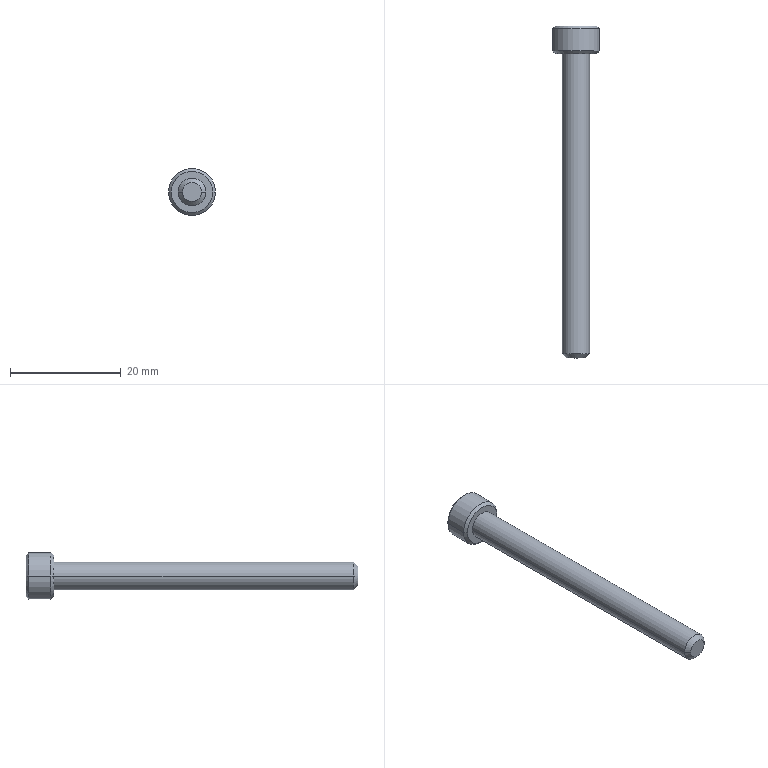Part | STEP file | BB62-M5-55L | 1 solid | 27 faces | box 8.5 x 60 x 8.5 mm | volume 1311 mm3 | plane 15 | cone 8 | cylinder 4 | commonest cylinder face diameters 5 x2 8.5 x2
STEP:
#1=CARTESIAN_POINT('',(0.,1.178,0.));
#2=VERTEX_POINT('',#1);
#3=CARTESIAN_POINT('',(2.29,2.5,0.));
#4=VERTEX_POINT('',#3);
#5=CARTESIAN_POINT('',(0.,1.178,0.));
#6=DIRECTION('',(0.866,0.5,0.));
#7=VECTOR('',#6,1000.);
#8=LINE('',#5,#7);
#9=EDGE_CURVE('',#2,#4,#8,.T.);
#10=ORIENTED_EDGE('',*,*,#9,.F.);
#11=CARTESIAN_POINT('',(-2.29,2.5,0.));
#12=VERTEX_POINT('',#11);
#13=CARTESIAN_POINT('',(0.,1.178,0.));
#14=DIRECTION('',(-0.866,0.5,0.));
#15=VECTOR('',#14,1000.);
#16=LINE('',#13,#15);
#17=EDGE_CURVE('',#2,#12,#16,.T.);
#18=ORIENTED_EDGE('',*,*,#17,.T.);
#19=CARTESIAN_POINT('',(-1.983,2.5,1.145));
#20=VERTEX_POINT('',#19);
#21=CARTESIAN_POINT('',(0.,2.5,0.));
#22=DIRECTION('',(0.,-1.,0.));
#23=DIRECTION('',(-1.,0.,0.));
#24=AXIS2_PLACEMENT_3D('',#21,#22,#23);
#25=CIRCLE('',#24,2.29);
#26=EDGE_CURVE('',#20,#12,#25,.T.);
#27=ORIENTED_EDGE('',*,*,#26,.F.);
#28=CARTESIAN_POINT('',(0.,2.5,2.29));
#29=VERTEX_POINT('',#28);
#30=CARTESIAN_POINT('',(0.,2.5,0.));
#31=DIRECTION('',(0.,-1.,0.));
#32=DIRECTION('',(-1.,0.,0.));
#33=AXIS2_PLACEMENT_3D('',#30,#31,#32);
#34=CIRCLE('',#33,2.29);
#35=EDGE_CURVE('',#29,#20,#34,.T.);
#36=ORIENTED_EDGE('',*,*,#35,.F.);
#37=CARTESIAN_POINT('',(1.983,2.5,1.145));
#38=VERTEX_POINT('',#37);
#39=CARTESIAN_POINT('',(0.,2.5,0.));
#40=DIRECTION('',(0.,-1.,0.));
#41=DIRECTION('',(-1.,0.,0.));
#42=AXIS2_PLACEMENT_3D('',#39,#40,#41);
#43=CIRCLE('',#42,2.29);
#44=EDGE_CURVE('',#38,#29,#43,.T.);
#45=ORIENTED_EDGE('',*,*,#44,.F.);
#46=CARTESIAN_POINT('',(0.,2.5,0.));
#47=DIRECTION('',(0.,-1.,0.));
#48=DIRECTION('',(-1.,0.,0.));
#49=AXIS2_PLACEMENT_3D('',#46,#47,#48);
#50=CIRCLE('',#49,2.29);
#51=EDGE_CURVE('',#4,#38,#50,.T.);
#52=ORIENTED_EDGE('',*,*,#51,.F.);
#53=EDGE_LOOP('',(#10,#18,#27,#36,#45,#52));
#54=FACE_OUTER_BOUND('',#53,.T.);
#55=CARTESIAN_POINT('',(0.,1001.178,0.));
#56=DIRECTION('',(0.,1.,0.));
#57=DIRECTION('',(1.,0.,0.));
#58=AXIS2_PLACEMENT_3D('',#55,#56,#57);
#59=CONICAL_SURFACE('',#58,1732.051,1.047);
#60=ADVANCED_FACE('',(#54),#59,.F.);
#61=CARTESIAN_POINT('',(1.7,-55.,0.));
#62=VERTEX_POINT('',#61);
#63=CARTESIAN_POINT('',(-1.7,-55.,0.));
#64=VERTEX_POINT('',#63);
#65=CARTESIAN_POINT('',(0.,-55.,0.));
#66=DIRECTION('',(0.,1.,0.));
#67=DIRECTION('',(1.,0.,0.));
#68=AXIS2_PLACEMENT_3D('',#65,#66,#67);
#69=CIRCLE('',#68,1.7);
#70=EDGE_CURVE('',#62,#64,#69,.T.);
#71=ORIENTED_EDGE('',*,*,#70,.T.);
#72=CARTESIAN_POINT('',(-2.5,-54.2,0.));
#73=VERTEX_POINT('',#72);
#74=CARTESIAN_POINT('',(-1.7,-55.,0.));
#75=DIRECTION('',(-0.7071,0.7071,0.));
#76=VECTOR('',#75,1000.);
#77=LINE('',#74,#76);
#78=EDGE_CURVE('',#64,#73,#77,.T.);
#79=ORIENTED_EDGE('',*,*,#78,.T.);
#80=CARTESIAN_POINT('',(2.5,-54.2,0.));
#81=VERTEX_POINT('',#80);
#82=CARTESIAN_POINT('',(0.,-54.2,0.));
#83=DIRECTION('',(0.,-1.,0.));
#84=DIRECTION('',(-1.,0.,0.));
#85=AXIS2_PLACEMENT_3D('',#82,#83,#84);
#86=CIRCLE('',#85,2.5);
#87=EDGE_CURVE('',#73,#81,#86,.T.);
#88=ORIENTED_EDGE('',*,*,#87,.T.);
#89=CARTESIAN_POINT('',(1.7,-55.,0.));
#90=DIRECTION('',(0.7071,0.7071,0.));
#91=VECTOR('',#90,1000.);
#92=LINE('',#89,#91);
#93=EDGE_CURVE('',#62,#81,#92,.T.);
#94=ORIENTED_EDGE('',*,*,#93,.F.);
#95=EDGE_LOOP('',(#71,#79,#88,#94));
#96=FACE_OUTER_BOUND('',#95,.T.);
#97=CARTESIAN_POINT('',(0.,-55.,0.));
#98=DIRECTION('',(0.,1.,0.));
#99=DIRECTION('',(1.,0.,0.));
#100=AXIS2_PLACEMENT_3D('',#97,#98,#99);
#101=CONICAL_SURFACE('',#100,1.7,0.7854);
#102=ADVANCED_FACE('',(#96),#101,.T.);
#103=ORIENTED_EDGE('',*,*,#87,.F.);
#104=CARTESIAN_POINT('',(-2.5,0.,0.));
#105=VERTEX_POINT('',#104);
#106=CARTESIAN_POINT('',(-2.5,-54.2,0.));
#107=DIRECTION('',(0.,1.,0.));
#108=VECTOR('',#107,1000.);
#109=LINE('',#106,#108);
#110=EDGE_CURVE('',#73,#105,#109,.T.);
#111=ORIENTED_EDGE('',*,*,#110,.T.);
#112=CARTESIAN_POINT('',(2.5,0.,0.));
#113=VERTEX_POINT('',#112);
#114=CARTESIAN_POINT('',(0.,0.,0.));
#115=DIRECTION('',(0.,-1.,0.));
#116=DIRECTION('',(-1.,0.,0.));
#117=AXIS2_PLACEMENT_3D('',#114,#115,#116);
#118=CIRCLE('',#117,2.5);
#119=EDGE_CURVE('',#105,#113,#118,.T.);
#120=ORIENTED_EDGE('',*,*,#119,.T.);
#121=CARTESIAN_POINT('',(2.5,-54.2,0.));
#122=DIRECTION('',(0.,1.,0.));
#123=VECTOR('',#122,1000.);
#124=LINE('',#121,#123);
#125=EDGE_CURVE('',#81,#113,#124,.T.);
#126=ORIENTED_EDGE('',*,*,#125,.F.);
#127=EDGE_LOOP('',(#103,#111,#120,#126));
#128=FACE_OUTER_BOUND('',#127,.T.);
#129=CARTESIAN_POINT('',(0.,-54.2,0.));
#130=DIRECTION('',(0.,1.,0.));
#131=DIRECTION('',(1.,0.,0.));
#132=AXIS2_PLACEMENT_3D('',#129,#130,#131);
#133=CYLINDRICAL_SURFACE('',#132,2.5);
#134=ADVANCED_FACE('',(#128),#133,.T.);
#135=CARTESIAN_POINT('',(-3.75,5.,0.));
#136=VERTEX_POINT('',#135);
#137=CARTESIAN_POINT('',(3.75,5.,0.));
#138=VERTEX_POINT('',#137);
#139=CARTESIAN_POINT('',(0.,5.,0.));
#140=DIRECTION('',(0.,-1.,0.));
#141=DIRECTION('',(-1.,0.,0.));
#142=AXIS2_PLACEMENT_3D('',#139,#140,#141);
#143=CIRCLE('',#142,3.75);
#144=EDGE_CURVE('',#136,#138,#143,.T.);
#145=ORIENTED_EDGE('',*,*,#144,.T.);
#146=CARTESIAN_POINT('',(4.25,4.5,0.));
#147=VERTEX_POINT('',#146);
#148=CARTESIAN_POINT('',(4.25,4.5,0.));
#149=DIRECTION('',(0.7071,-0.7071,0.));
#150=VECTOR('',#149,1000.);
#151=LINE('',#148,#150);
#152=EDGE_CURVE('',#138,#147,#151,.T.);
#153=ORIENTED_EDGE('',*,*,#152,.T.);
#154=CARTESIAN_POINT('',(-4.25,4.5,0.));
#155=VERTEX_POINT('',#154);
#156=CARTESIAN_POINT('',(0.,4.5,0.));
#157=DIRECTION('',(0.,-1.,0.));
#158=DIRECTION('',(-1.,0.,0.));
#159=AXIS2_PLACEMENT_3D('',#156,#157,#158);
#160=CIRCLE('',#159,4.25);
#161=EDGE_CURVE('',#155,#147,#160,.T.);
#162=ORIENTED_EDGE('',*,*,#161,.F.);
#163=CARTESIAN_POINT('',(-4.25,4.5,0.));
#164=DIRECTION('',(-0.7071,-0.7071,0.));
#165=VECTOR('',#164,1000.);
#166=LINE('',#163,#165);
#167=EDGE_CURVE('',#136,#155,#166,.T.);
#168=ORIENTED_EDGE('',*,*,#167,.F.);
#169=EDGE_LOOP('',(#145,#153,#162,#168));
#170=FACE_OUTER_BOUND('',#169,.T.);
#171=CARTESIAN_POINT('',(0.,4.5,0.));
#172=DIRECTION('',(0.,-1.,0.));
#173=DIRECTION('',(-1.,0.,0.));
#174=AXIS2_PLACEMENT_3D('',#171,#172,#173);
#175=CONICAL_SURFACE('',#174,4.25,0.7854);
#176=ADVANCED_FACE('',(#170),#175,.T.);
#177=ORIENTED_EDGE('',*,*,#161,.T.);
#178=CARTESIAN_POINT('',(4.25,0.5,0.));
#179=VERTEX_POINT('',#178);
#180=CARTESIAN_POINT('',(4.25,1.62,0.));
#181=DIRECTION('',(0.,-1.,0.));
#182=VECTOR('',#181,1000.);
#183=LINE('',#180,#182);
#184=EDGE_CURVE('',#147,#179,#183,.T.);
#185=ORIENTED_EDGE('',*,*,#184,.T.);
#186=CARTESIAN_POINT('',(-4.25,0.5,0.));
#187=VERTEX_POINT('',#186);
#188=CARTESIAN_POINT('',(0.,0.5,0.));
#189=DIRECTION('',(0.,-1.,0.));
#190=DIRECTION('',(-1.,0.,0.));
#191=AXIS2_PLACEMENT_3D('',#188,#189,#190);
#192=CIRCLE('',#191,4.25);
#193=EDGE_CURVE('',#187,#179,#192,.T.);
#194=ORIENTED_EDGE('',*,*,#193,.F.);
#195=CARTESIAN_POINT('',(-4.25,1.62,0.));
#196=DIRECTION('',(0.,-1.,0.));
#197=VECTOR('',#196,1000.);
#198=LINE('',#195,#197);
#199=EDGE_CURVE('',#155,#187,#198,.T.);
#200=ORIENTED_EDGE('',*,*,#199,.F.);
#201=EDGE_LOOP('',(#177,#185,#194,#200));
#202=FACE_OUTER_BOUND('',#201,.T.);
#203=CARTESIAN_POINT('',(0.,1.62,0.));
#204=DIRECTION('',(0.,-1.,0.));
#205=DIRECTION('',(-1.,0.,0.));
#206=AXIS2_PLACEMENT_3D('',#203,#204,#205);
#207=CYLINDRICAL_SURFACE('',#206,4.25);
#208=ADVANCED_FACE('',(#202),#207,.T.);
#209=CARTESIAN_POINT('',(-3.75,0.,0.));
#210=VERTEX_POINT('',#209);
#211=CARTESIAN_POINT('',(3.75,0.,0.));
#212=VERTEX_POINT('',#211);
#213=CARTESIAN_POINT('',(0.,0.,0.));
#214=DIRECTION('',(0.,-1.,0.));
#215=DIRECTION('',(-1.,0.,0.));
#216=AXIS2_PLACEMENT_3D('',#213,#214,#215);
#217=CIRCLE('',#216,3.75);
#218=EDGE_CURVE('',#210,#212,#217,.T.);
#219=ORIENTED_EDGE('',*,*,#218,.F.);
#220=CARTESIAN_POINT('',(-3.75,0.,0.));
#221=DIRECTION('',(-0.7071,0.7071,0.));
#222=VECTOR('',#221,1000.);
#223=LINE('',#220,#222);
#224=EDGE_CURVE('',#210,#187,#223,.T.);
#225=ORIENTED_EDGE('',*,*,#224,.T.);
#226=ORIENTED_EDGE('',*,*,#193,.T.);
#227=CARTESIAN_POINT('',(3.75,0.,0.));
#228=DIRECTION('',(0.7071,0.7071,0.));
#229=VECTOR('',#228,1000.);
#230=LINE('',#227,#229);
#231=EDGE_CURVE('',#212,#179,#230,.T.);
#232=ORIENTED_EDGE('',*,*,#231,.F.);
#233=EDGE_LOOP('',(#219,#225,#226,#232));
#234=FACE_OUTER_BOUND('',#233,.T.);
#235=CARTESIAN_POINT('',(0.,0.,0.));
#236=DIRECTION('',(0.,1.,0.));
#237=DIRECTION('',(1.,0.,0.));
#238=AXIS2_PLACEMENT_3D('',#235,#236,#237);
#239=CONICAL_SURFACE('',#238,3.75,0.7854);
#240=ADVANCED_FACE('',(#234),#239,.T.);
#241=ORIENTED_EDGE('',*,*,#144,.F.);
#242=CARTESIAN_POINT('',(0.,5.,0.));
#243=DIRECTION('',(0.,-1.,0.));
#244=DIRECTION('',(-1.,0.,0.));
#245=AXIS2_PLACEMENT_3D('',#242,#243,#244);
#246=CIRCLE('',#245,3.75);
#247=EDGE_CURVE('',#138,#136,#246,.T.);
#248=ORIENTED_EDGE('',*,*,#247,.F.);
#249=EDGE_LOOP('',(#241,#248));
#250=FACE_OUTER_BOUND('',#249,.T.);
#251=CARTESIAN_POINT('',(0.,5.,-2.29));
#252=VERTEX_POINT('',#251);
#253=CARTESIAN_POINT('',(-1.983,5.,-1.145));
#254=VERTEX_POINT('',#253);
#255=CARTESIAN_POINT('',(0.,5.,-2.29));
#256=DIRECTION('',(-0.866,0.,0.5));
#257=VECTOR('',#256,1000.);
#258=LINE('',#255,#257);
#259=EDGE_CURVE('',#252,#254,#258,.T.);
#260=ORIENTED_EDGE('',*,*,#259,.F.);
#261=CARTESIAN_POINT('',(1.983,5.,-1.145));
#262=VERTEX_POINT('',#261);
#263=CARTESIAN_POINT('',(1.983,5.,-1.145));
#264=DIRECTION('',(-0.866,0.,-0.5));
#265=VECTOR('',#264,1000.);
#266=LINE('',#263,#265);
#267=EDGE_CURVE('',#262,#252,#266,.T.);
#268=ORIENTED_EDGE('',*,*,#267,.F.);
#269=CARTESIAN_POINT('',(1.983,5.,1.145));
#270=VERTEX_POINT('',#269);
#271=CARTESIAN_POINT('',(1.983,5.,1.145));
#272=DIRECTION('',(0.,0.,-1.));
#273=VECTOR('',#272,1000.);
#274=LINE('',#271,#273);
#275=EDGE_CURVE('',#270,#262,#274,.T.);
#276=ORIENTED_EDGE('',*,*,#275,.F.);
#277=CARTESIAN_POINT('',(0.,5.,2.29));
#278=VERTEX_POINT('',#277);
#279=CARTESIAN_POINT('',(0.,5.,2.29));
#280=DIRECTION('',(0.866,0.,-0.5));
#281=VECTOR('',#280,1000.);
#282=LINE('',#279,#281);
#283=EDGE_CURVE('',#278,#270,#282,.T.);
#284=ORIENTED_EDGE('',*,*,#283,.F.);
#285=CARTESIAN_POINT('',(-1.983,5.,1.145));
#286=VERTEX_POINT('',#285);
#287=CARTESIAN_POINT('',(-1.983,5.,1.145));
#288=DIRECTION('',(0.866,0.,0.5));
#289=VECTOR('',#288,1000.);
#290=LINE('',#287,#289);
#291=EDGE_CURVE('',#286,#278,#290,.T.);
#292=ORIENTED_EDGE('',*,*,#291,.F.);
#293=CARTESIAN_POINT('',(-1.983,5.,-1.145));
#294=DIRECTION('',(0.,0.,1.));
#295=VECTOR('',#294,1000.);
#296=LINE('',#293,#295);
#297=EDGE_CURVE('',#254,#286,#296,.T.);
#298=ORIENTED_EDGE('',*,*,#297,.F.);
#299=EDGE_LOOP('',(#260,#268,#276,#284,#292,#298));
#300=FACE_BOUND('',#299,.T.);
#301=CARTESIAN_POINT('',(3.75,5.,0.));
#302=DIRECTION('',(0.,1.,0.));
#303=DIRECTION('',(1.,0.,0.));
#304=AXIS2_PLACEMENT_3D('',#301,#302,#303);
#305=PLANE('',#304);
#306=ADVANCED_FACE('',(#250,#300),#305,.T.);
#307=CARTESIAN_POINT('',(0.,0.,0.));
#308=DIRECTION('',(0.,-1.,0.));
#309=DIRECTION('',(-1.,0.,0.));
#310=AXIS2_PLACEMENT_3D('',#307,#308,#309);
#311=CIRCLE('',#310,2.5);
#312=EDGE_CURVE('',#113,#105,#311,.T.);
#313=ORIENTED_EDGE('',*,*,#312,.F.);
#314=ORIENTED_EDGE('',*,*,#119,.F.);
#315=EDGE_LOOP('',(#313,#314));
#316=FACE_BOUND('',#315,.T.);
#317=CARTESIAN_POINT('',(0.,0.,0.));
#318=DIRECTION('',(0.,-1.,0.));
#319=DIRECTION('',(-1.,0.,0.));
#320=AXIS2_PLACEMENT_3D('',#317,#318,#319);
#321=CIRCLE('',#320,3.75);
#322=EDGE_CURVE('',#212,#210,#321,.T.);
#323=ORIENTED_EDGE('',*,*,#322,.T.);
#324=ORIENTED_EDGE('',*,*,#218,.T.);
#325=EDGE_LOOP('',(#323,#324));
#326=FACE_OUTER_BOUND('',#325,.T.);
#327=CARTESIAN_POINT('',(0.,0.,0.));
#328=DIRECTION('',(0.,-1.,0.));
#329=DIRECTION('',(-1.,0.,0.));
#330=AXIS2_PLACEMENT_3D('',#327,#328,#329);
#331=PLANE('',#330);
#332=ADVANCED_FACE('',(#316,#326),#331,.T.);
#333=ORIENTED_EDGE('',*,*,#224,.F.);
#334=ORIENTED_EDGE('',*,*,#322,.F.);
#335=ORIENTED_EDGE('',*,*,#231,.T.);
#336=CARTESIAN_POINT('',(0.,0.5,0.));
#337=DIRECTION('',(0.,-1.,0.));
#338=DIRECTION('',(-1.,0.,0.));
#339=AXIS2_PLACEMENT_3D('',#336,#337,#338);
#340=CIRCLE('',#339,4.25);
#341=EDGE_CURVE('',#179,#187,#340,.T.);
#342=ORIENTED_EDGE('',*,*,#341,.T.);
#343=EDGE_LOOP('',(#333,#334,#335,#342));
#344=FACE_OUTER_BOUND('',#343,.T.);
#345=CARTESIAN_POINT('',(0.,0.,0.));
#346=DIRECTION('',(0.,1.,0.));
#347=DIRECTION('',(1.,0.,0.));
#348=AXIS2_PLACEMENT_3D('',#345,#346,#347);
#349=CONICAL_SURFACE('',#348,3.75,0.7854);
#350=ADVANCED_FACE('',(#344),#349,.T.);
#351=ORIENTED_EDGE('',*,*,#184,.F.);
#352=CARTESIAN_POINT('',(0.,4.5,0.));
#353=DIRECTION('',(0.,-1.,0.));
#354=DIRECTION('',(-1.,0.,0.));
#355=AXIS2_PLACEMENT_3D('',#352,#353,#354);
#356=CIRCLE('',#355,4.25);
#357=EDGE_CURVE('',#147,#155,#356,.T.);
#358=ORIENTED_EDGE('',*,*,#357,.T.);
#359=ORIENTED_EDGE('',*,*,#199,.T.);
#360=ORIENTED_EDGE('',*,*,#341,.F.);
#361=EDGE_LOOP('',(#351,#358,#359,#360));
#362=FACE_OUTER_BOUND('',#361,.T.);
#363=CARTESIAN_POINT('',(0.,1.62,0.));
#364=DIRECTION('',(0.,-1.,0.));
#365=DIRECTION('',(-1.,0.,0.));
#366=AXIS2_PLACEMENT_3D('',#363,#364,#365);
#367=CYLINDRICAL_SURFACE('',#366,4.25);
#368=ADVANCED_FACE('',(#362),#367,.T.);
#369=ORIENTED_EDGE('',*,*,#152,.F.);
#370=ORIENTED_EDGE('',*,*,#247,.T.);
#371=ORIENTED_EDGE('',*,*,#167,.T.);
#372=ORIENTED_EDGE('',*,*,#357,.F.);
#373=EDGE_LOOP('',(#369,#370,#371,#372));
#374=FACE_OUTER_BOUND('',#373,.T.);
#375=CARTESIAN_POINT('',(0.,4.5,0.));
#376=DIRECTION('',(0.,-1.,0.));
#377=DIRECTION('',(-1.,0.,0.));
#378=AXIS2_PLACEMENT_3D('',#375,#376,#377);
#379=CONICAL_SURFACE('',#378,4.25,0.7854);
#380=ADVANCED_FACE('',(#374),#379,.T.);
#381=ORIENTED_EDGE('',*,*,#110,.F.);
#382=CARTESIAN_POINT('',(0.,-54.2,0.));
#383=DIRECTION('',(0.,-1.,0.));
#384=DIRECTION('',(-1.,0.,0.));
#385=AXIS2_PLACEMENT_3D('',#382,#383,#384);
#386=CIRCLE('',#385,2.5);
#387=EDGE_CURVE('',#81,#73,#386,.T.);
#388=ORIENTED_EDGE('',*,*,#387,.F.);
#389=ORIENTED_EDGE('',*,*,#125,.T.);
#390=ORIENTED_EDGE('',*,*,#312,.T.);
#391=EDGE_LOOP('',(#381,#388,#389,#390));
#392=FACE_OUTER_BOUND('',#391,.T.);
#393=CARTESIAN_POINT('',(0.,-54.2,0.));
#394=DIRECTION('',(0.,1.,0.));
#395=DIRECTION('',(1.,0.,0.));
#396=AXIS2_PLACEMENT_3D('',#393,#394,#395);
#397=CYLINDRICAL_SURFACE('',#396,2.5);
#398=ADVANCED_FACE('',(#392),#397,.T.);
#399=ORIENTED_EDGE('',*,*,#70,.F.);
#400=CARTESIAN_POINT('',(0.,-55.,0.));
#401=DIRECTION('',(0.,1.,0.));
#402=DIRECTION('',(1.,0.,0.));
#403=AXIS2_PLACEMENT_3D('',#400,#401,#402);
#404=CIRCLE('',#403,1.7);
#405=EDGE_CURVE('',#64,#62,#404,.T.);
#406=ORIENTED_EDGE('',*,*,#405,.F.);
#407=EDGE_LOOP('',(#399,#406));
#408=FACE_OUTER_BOUND('',#407,.T.);
#409=CARTESIAN_POINT('',(0.,-55.,0.));
#410=DIRECTION('',(0.,-1.,0.));
#411=DIRECTION('',(-1.,0.,0.));
#412=AXIS2_PLACEMENT_3D('',#409,#410,#411);
#413=PLANE('',#412);
#414=ADVANCED_FACE('',(#408),#413,.T.);
#415=ORIENTED_EDGE('',*,*,#78,.F.);
#416=ORIENTED_EDGE('',*,*,#405,.T.);
#417=ORIENTED_EDGE('',*,*,#93,.T.);
#418=ORIENTED_EDGE('',*,*,#387,.T.);
#419=EDGE_LOOP('',(#415,#416,#417,#418));
#420=FACE_OUTER_BOUND('',#419,.T.);
#421=CARTESIAN_POINT('',(0.,-55.,0.));
#422=DIRECTION('',(0.,1.,0.));
#423=DIRECTION('',(1.,0.,0.));
#424=AXIS2_PLACEMENT_3D('',#421,#422,#423);
#425=CONICAL_SURFACE('',#424,1.7,0.7854);
#426=ADVANCED_FACE('',(#420),#425,.T.);
#427=CARTESIAN_POINT('',(1.983,2.5,-1.145));
#428=VERTEX_POINT('',#427);
#429=CARTESIAN_POINT('',(0.,2.5,-2.29));
#430=VERTEX_POINT('',#429);
#431=CARTESIAN_POINT('',(1.983,2.5,-1.145));
#432=DIRECTION('',(-0.866,0.,-0.5));
#433=VECTOR('',#432,1000.);
#434=LINE('',#431,#433);
#435=EDGE_CURVE('',#428,#430,#434,.T.);
#436=ORIENTED_EDGE('',*,*,#435,.F.);
#437=CARTESIAN_POINT('',(1.983,5.,-1.145));
#438=DIRECTION('',(0.,-1.,0.));
#439=VECTOR('',#438,1000.);
#440=LINE('',#437,#439);
#441=EDGE_CURVE('',#262,#428,#440,.T.);
#442=ORIENTED_EDGE('',*,*,#441,.F.);
#443=ORIENTED_EDGE('',*,*,#267,.T.);
#444=CARTESIAN_POINT('',(0.,5.,-2.29));
#445=DIRECTION('',(0.,-1.,0.));
#446=VECTOR('',#445,1000.);
#447=LINE('',#444,#446);
#448=EDGE_CURVE('',#252,#430,#447,.T.);
#449=ORIENTED_EDGE('',*,*,#448,.T.);
#450=EDGE_LOOP('',(#436,#442,#443,#449));
#451=FACE_OUTER_BOUND('',#450,.T.);
#452=CARTESIAN_POINT('',(1.983,5.,-1.145));
#453=DIRECTION('',(-0.5,0.,0.866));
#454=DIRECTION('',(0.866,0.,0.5));
#455=AXIS2_PLACEMENT_3D('',#452,#453,#454);
#456=PLANE('',#455);
#457=ADVANCED_FACE('',(#451),#456,.T.);
#458=CARTESIAN_POINT('',(-1.983,2.5,-1.145));
#459=VERTEX_POINT('',#458);
#460=CARTESIAN_POINT('',(0.,2.5,-2.29));
#461=DIRECTION('',(-0.866,0.,0.5));
#462=VECTOR('',#461,1000.);
#463=LINE('',#460,#462);
#464=EDGE_CURVE('',#430,#459,#463,.T.);
#465=ORIENTED_EDGE('',*,*,#464,.F.);
#466=ORIENTED_EDGE('',*,*,#448,.F.);
#467=ORIENTED_EDGE('',*,*,#259,.T.);
#468=CARTESIAN_POINT('',(-1.983,5.,-1.145));
#469=DIRECTION('',(0.,-1.,0.));
#470=VECTOR('',#469,1000.);
#471=LINE('',#468,#470);
#472=EDGE_CURVE('',#254,#459,#471,.T.);
#473=ORIENTED_EDGE('',*,*,#472,.T.);
#474=EDGE_LOOP('',(#465,#466,#467,#473));
#475=FACE_OUTER_BOUND('',#474,.T.);
#476=CARTESIAN_POINT('',(0.,5.,-2.29));
#477=DIRECTION('',(0.5,0.,0.866));
#478=DIRECTION('',(0.866,0.,-0.5));
#479=AXIS2_PLACEMENT_3D('',#476,#477,#478);
#480=PLANE('',#479);
#481=ADVANCED_FACE('',(#475),#480,.T.);
#482=CARTESIAN_POINT('',(-1.983,2.5,-1.145));
#483=DIRECTION('',(0.,0.,1.));
#484=VECTOR('',#483,1000.);
#485=LINE('',#482,#484);
#486=EDGE_CURVE('',#459,#20,#485,.T.);
#487=ORIENTED_EDGE('',*,*,#486,.F.);
#488=ORIENTED_EDGE('',*,*,#472,.F.);
#489=ORIENTED_EDGE('',*,*,#297,.T.);
#490=CARTESIAN_POINT('',(-1.983,5.,1.145));
#491=DIRECTION('',(0.,-1.,0.));
#492=VECTOR('',#491,1000.);
#493=LINE('',#490,#492);
#494=EDGE_CURVE('',#286,#20,#493,.T.);
#495=ORIENTED_EDGE('',*,*,#494,.T.);
#496=EDGE_LOOP('',(#487,#488,#489,#495));
#497=FACE_OUTER_BOUND('',#496,.T.);
#498=CARTESIAN_POINT('',(-1.983,5.,-1.145));
#499=DIRECTION('',(1.,0.,0.));
#500=DIRECTION('',(0.,0.,-1.));
#501=AXIS2_PLACEMENT_3D('',#498,#499,#500);
#502=PLANE('',#501);
#503=ADVANCED_FACE('',(#497),#502,.T.);
#504=CARTESIAN_POINT('',(-1.983,2.5,1.145));
#505=DIRECTION('',(0.866,0.,0.5));
#506=VECTOR('',#505,1000.);
#507=LINE('',#504,#506);
#508=EDGE_CURVE('',#20,#29,#507,.T.);
#509=ORIENTED_EDGE('',*,*,#508,.F.);
#510=ORIENTED_EDGE('',*,*,#494,.F.);
#511=ORIENTED_EDGE('',*,*,#291,.T.);
#512=CARTESIAN_POINT('',(0.,5.,2.29));
#513=DIRECTION('',(0.,-1.,0.));
#514=VECTOR('',#513,1000.);
#515=LINE('',#512,#514);
#516=EDGE_CURVE('',#278,#29,#515,.T.);
#517=ORIENTED_EDGE('',*,*,#516,.T.);
#518=EDGE_LOOP('',(#509,#510,#511,#517));
#519=FACE_OUTER_BOUND('',#518,.T.);
#520=CARTESIAN_POINT('',(-1.983,5.,1.145));
#521=DIRECTION('',(0.5,0.,-0.866));
#522=DIRECTION('',(-0.866,0.,-0.5));
#523=AXIS2_PLACEMENT_3D('',#520,#521,#522);
#524=PLANE('',#523);
#525=ADVANCED_FACE('',(#519),#524,.T.);
#526=CARTESIAN_POINT('',(0.,2.5,2.29));
#527=DIRECTION('',(0.866,0.,-0.5));
#528=VECTOR('',#527,1000.);
#529=LINE('',#526,#528);
#530=EDGE_CURVE('',#29,#38,#529,.T.);
#531=ORIENTED_EDGE('',*,*,#530,.F.);
#532=ORIENTED_EDGE('',*,*,#516,.F.);
#533=ORIENTED_EDGE('',*,*,#283,.T.);
#534=CARTESIAN_POINT('',(1.983,5.,1.145));
#535=DIRECTION('',(0.,-1.,0.));
#536=VECTOR('',#535,1000.);
#537=LINE('',#534,#536);
#538=EDGE_CURVE('',#270,#38,#537,.T.);
#539=ORIENTED_EDGE('',*,*,#538,.T.);
#540=EDGE_LOOP('',(#531,#532,#533,#539));
#541=FACE_OUTER_BOUND('',#540,.T.);
#542=CARTESIAN_POINT('',(0.,5.,2.29));
#543=DIRECTION('',(-0.5,0.,-0.866));
#544=DIRECTION('',(-0.866,0.,0.5));
#545=AXIS2_PLACEMENT_3D('',#542,#543,#544);
#546=PLANE('',#545);
#547=ADVANCED_FACE('',(#541),#546,.T.);
#548=CARTESIAN_POINT('',(1.983,2.5,1.145));
#549=DIRECTION('',(0.,0.,-1.));
#550=VECTOR('',#549,1000.);
#551=LINE('',#548,#550);
#552=EDGE_CURVE('',#38,#428,#551,.T.);
#553=ORIENTED_EDGE('',*,*,#552,.F.);
#554=ORIENTED_EDGE('',*,*,#538,.F.);
#555=ORIENTED_EDGE('',*,*,#275,.T.);
#556=ORIENTED_EDGE('',*,*,#441,.T.);
#557=EDGE_LOOP('',(#553,#554,#555,#556));
#558=FACE_OUTER_BOUND('',#557,.T.);
#559=CARTESIAN_POINT('',(1.983,5.,1.145));
#560=DIRECTION('',(-1.,0.,0.));
#561=DIRECTION('',(0.,0.,1.));
#562=AXIS2_PLACEMENT_3D('',#559,#560,#561);
#563=PLANE('',#562);
#564=ADVANCED_FACE('',(#558),#563,.T.);
#565=ORIENTED_EDGE('',*,*,#435,.T.);
#566=CARTESIAN_POINT('',(0.,2.5,0.));
#567=DIRECTION('',(0.,-1.,0.));
#568=DIRECTION('',(-1.,0.,0.));
#569=AXIS2_PLACEMENT_3D('',#566,#567,#568);
#570=CIRCLE('',#569,2.29);
#571=EDGE_CURVE('',#430,#428,#570,.T.);
#572=ORIENTED_EDGE('',*,*,#571,.T.);
#573=EDGE_LOOP('',(#565,#572));
#574=FACE_OUTER_BOUND('',#573,.T.);
#575=CARTESIAN_POINT('',(0.,2.5,0.));
#576=DIRECTION('',(0.,1.,0.));
#577=DIRECTION('',(1.,0.,0.));
#578=AXIS2_PLACEMENT_3D('',#575,#576,#577);
#579=PLANE('',#578);
#580=ADVANCED_FACE('',(#574),#579,.F.);
#581=ORIENTED_EDGE('',*,*,#552,.T.);
#582=CARTESIAN_POINT('',(0.,2.5,0.));
#583=DIRECTION('',(0.,-1.,0.));
#584=DIRECTION('',(-1.,0.,0.));
#585=AXIS2_PLACEMENT_3D('',#582,#583,#584);
#586=CIRCLE('',#585,2.29);
#587=EDGE_CURVE('',#428,#4,#586,.T.);
#588=ORIENTED_EDGE('',*,*,#587,.T.);
#589=ORIENTED_EDGE('',*,*,#51,.T.);
#590=EDGE_LOOP('',(#581,#588,#589));
#591=FACE_OUTER_BOUND('',#590,.T.);
#592=CARTESIAN_POINT('',(0.,2.5,0.));
#593=DIRECTION('',(0.,1.,0.));
#594=DIRECTION('',(1.,0.,0.));
#595=AXIS2_PLACEMENT_3D('',#592,#593,#594);
#596=PLANE('',#595);
#597=ADVANCED_FACE('',(#591),#596,.F.);
#598=ORIENTED_EDGE('',*,*,#530,.T.);
#599=ORIENTED_EDGE('',*,*,#44,.T.);
#600=EDGE_LOOP('',(#598,#599));
#601=FACE_OUTER_BOUND('',#600,.T.);
#602=CARTESIAN_POINT('',(0.,2.5,0.));
#603=DIRECTION('',(0.,1.,0.));
#604=DIRECTION('',(1.,0.,0.));
#605=AXIS2_PLACEMENT_3D('',#602,#603,#604);
#606=PLANE('',#605);
#607=ADVANCED_FACE('',(#601),#606,.F.);
#608=ORIENTED_EDGE('',*,*,#508,.T.);
#609=ORIENTED_EDGE('',*,*,#35,.T.);
#610=EDGE_LOOP('',(#608,#609));
#611=FACE_OUTER_BOUND('',#610,.T.);
#612=CARTESIAN_POINT('',(0.,2.5,0.));
#613=DIRECTION('',(0.,1.,0.));
#614=DIRECTION('',(1.,0.,0.));
#615=AXIS2_PLACEMENT_3D('',#612,#613,#614);
#616=PLANE('',#615);
#617=ADVANCED_FACE('',(#611),#616,.F.);
#618=ORIENTED_EDGE('',*,*,#486,.T.);
#619=ORIENTED_EDGE('',*,*,#26,.T.);
#620=CARTESIAN_POINT('',(0.,2.5,0.));
#621=DIRECTION('',(0.,-1.,0.));
#622=DIRECTION('',(-1.,0.,0.));
#623=AXIS2_PLACEMENT_3D('',#620,#621,#622);
#624=CIRCLE('',#623,2.29);
#625=EDGE_CURVE('',#12,#459,#624,.T.);
#626=ORIENTED_EDGE('',*,*,#625,.T.);
#627=EDGE_LOOP('',(#618,#619,#626));
#628=FACE_OUTER_BOUND('',#627,.T.);
#629=CARTESIAN_POINT('',(0.,2.5,0.));
#630=DIRECTION('',(0.,1.,0.));
#631=DIRECTION('',(1.,0.,0.));
#632=AXIS2_PLACEMENT_3D('',#629,#630,#631);
#633=PLANE('',#632);
#634=ADVANCED_FACE('',(#628),#633,.F.);
#635=ORIENTED_EDGE('',*,*,#464,.T.);
#636=CARTESIAN_POINT('',(0.,2.5,0.));
#637=DIRECTION('',(0.,-1.,0.));
#638=DIRECTION('',(-1.,0.,0.));
#639=AXIS2_PLACEMENT_3D('',#636,#637,#638);
#640=CIRCLE('',#639,2.29);
#641=EDGE_CURVE('',#459,#430,#640,.T.);
#642=ORIENTED_EDGE('',*,*,#641,.T.);
#643=EDGE_LOOP('',(#635,#642));
#644=FACE_OUTER_BOUND('',#643,.T.);
#645=CARTESIAN_POINT('',(0.,2.5,0.));
#646=DIRECTION('',(0.,1.,0.));
#647=DIRECTION('',(1.,0.,0.));
#648=AXIS2_PLACEMENT_3D('',#645,#646,#647);
#649=PLANE('',#648);
#650=ADVANCED_FACE('',(#644),#649,.F.);
#651=ORIENTED_EDGE('',*,*,#17,.F.);
#652=ORIENTED_EDGE('',*,*,#9,.T.);
#653=ORIENTED_EDGE('',*,*,#587,.F.);
#654=ORIENTED_EDGE('',*,*,#571,.F.);
#655=ORIENTED_EDGE('',*,*,#641,.F.);
#656=ORIENTED_EDGE('',*,*,#625,.F.);
#657=EDGE_LOOP('',(#651,#652,#653,#654,#655,#656));
#658=FACE_OUTER_BOUND('',#657,.T.);
#659=CARTESIAN_POINT('',(0.,1001.178,0.));
#660=DIRECTION('',(0.,1.,0.));
#661=DIRECTION('',(1.,0.,0.));
#662=AXIS2_PLACEMENT_3D('',#659,#660,#661);
#663=CONICAL_SURFACE('',#662,1732.051,1.047);
#664=ADVANCED_FACE('',(#658),#663,.F.);
#665=CLOSED_SHELL('',(#60,#102,#134,#176,#208,#240,#306,#332,#350,#368,#380,#398,#414,#426,#457,#481,#503,#525,#547,#564,#580,#597,#607,#617,#634,#650,#664));
#666=MANIFOLD_SOLID_BREP('',#665);
#667=CARTESIAN_POINT('',(0.,0.,0.));
#668=DIRECTION('',(0.,0.,1.));
#669=DIRECTION('',(1.,0.,0.));
#670=AXIS2_PLACEMENT_3D('',#667,#668,#669);
#671=(LENGTH_UNIT()NAMED_UNIT(*)SI_UNIT(.MILLI.,.METRE.));
#672=UNCERTAINTY_MEASURE_WITH_UNIT(LENGTH_MEASURE(0.00001),#671,'','');
#673=(NAMED_UNIT(*)PLANE_ANGLE_UNIT()SI_UNIT($,.RADIAN.));
#674=(NAMED_UNIT(*)SI_UNIT($,.STERADIAN.)SOLID_ANGLE_UNIT());
#675=(GEOMETRIC_REPRESENTATION_CONTEXT(3)GLOBAL_UNCERTAINTY_ASSIGNED_CONTEXT((#672))GLOBAL_UNIT_ASSIGNED_CONTEXT((#671,#673,#674))REPRESENTATION_CONTEXT('',''));
#676=ADVANCED_BREP_SHAPE_REPRESENTATION('',(#666,#670),#675);